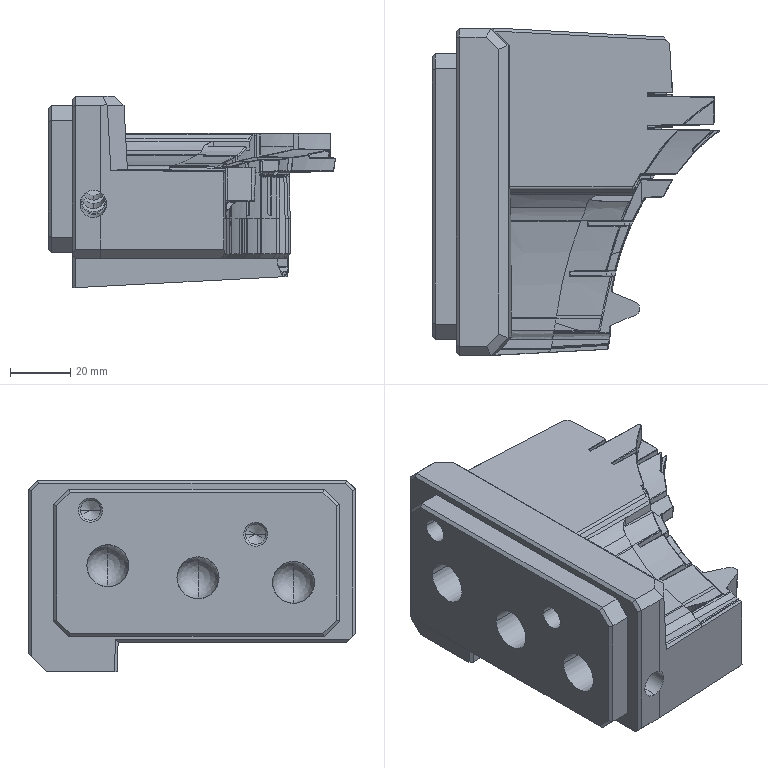Part | Creo | 1 solid | 895 faces | box 95.579 x 109 x 63.784 mm | volume 305519 mm3 | cylinder 325 | plane 257 | spline 130 | sphere 109 | other 37 | cone 33 | torus 4 | commonest cylinder face diameters 0.402 x228 0.804 x14 4.02 x11 8 x10 14 x6 1.006 x4